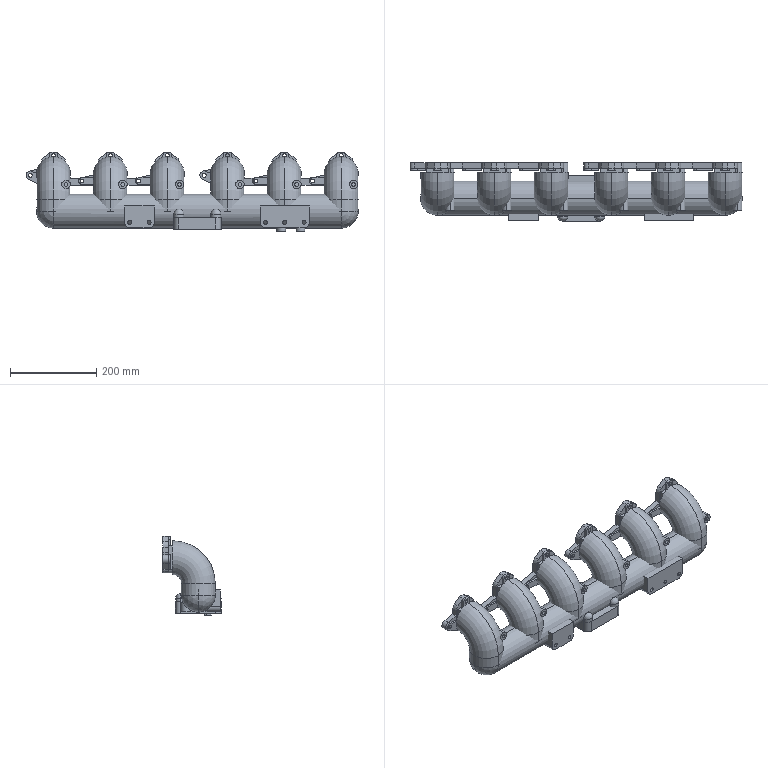Part | SolidWorks | features BaseBody 59 | 59 solids | 557 faces | box 771.5 x 135 x 185 mm | volume 5574936 mm3 | plane 311 | cylinder 210 | torus 24 | sphere 12 | commonest cylinder face diameters 9 x98 20 x34 50 x14 79 x14 10 x12 32 x12